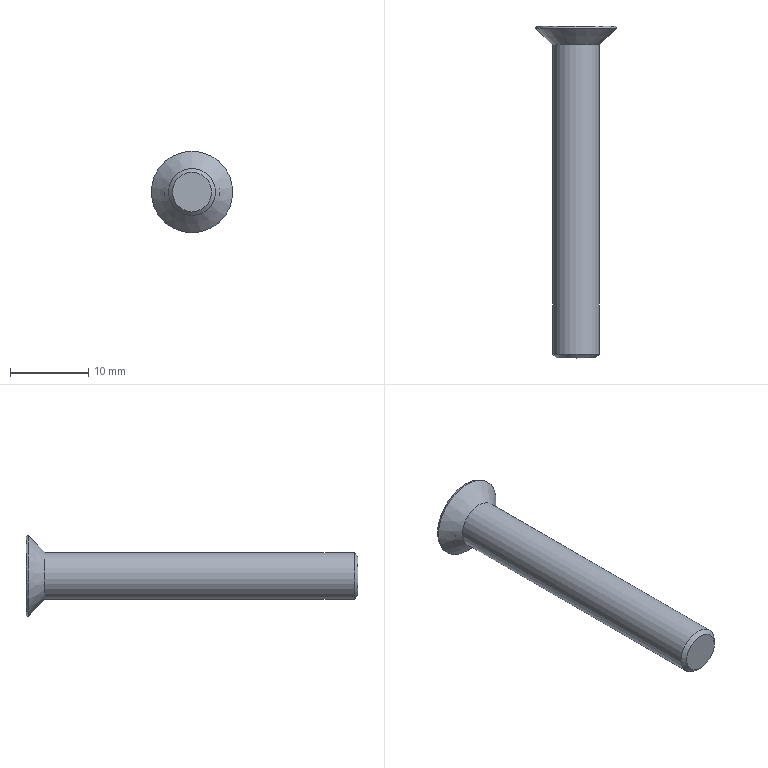Part | STEP file | SD30640 | 1 solid | 23 faces | box 10.421 x 42.38 x 10.421 mm | volume 1245 mm3 | plane 15 | cylinder 5 | cone 3 | commonest cylinder face diameters 0.4 x4 6 x1
STEP:
#1=CARTESIAN_POINT('',(0.,1.224,5.21));
#2=VERTEX_POINT('',#1);
#3=CARTESIAN_POINT('',(0.,1.224,0.));
#4=DIRECTION('',(0.,1.,0.));
#5=DIRECTION('',(0.,0.,1.));
#6=AXIS2_PLACEMENT_3D('',#3,#4,#5);
#7=CIRCLE('',#6,5.21);
#8=EDGE_CURVE('',#2,#2,#7,.T.);
#9=ORIENTED_EDGE('',*,*,#8,.F.);
#10=EDGE_LOOP('',(#9));
#11=FACE_OUTER_BOUND('',#10,.T.);
#12=CARTESIAN_POINT('',(0.,-0.88,-3.));
#13=VERTEX_POINT('',#12);
#14=CARTESIAN_POINT('',(0.,-0.88,0.));
#15=DIRECTION('',(0.,-1.,0.));
#16=DIRECTION('',(0.,0.,-1.));
#17=AXIS2_PLACEMENT_3D('',#14,#15,#16);
#18=CIRCLE('',#17,3.);
#19=EDGE_CURVE('',#13,#13,#18,.T.);
#20=ORIENTED_EDGE('',*,*,#19,.F.);
#21=EDGE_LOOP('',(#20));
#22=FACE_BOUND('',#21,.T.);
#23=CARTESIAN_POINT('',(0.,-0.88,0.));
#24=DIRECTION('',(0.,1.,0.));
#25=DIRECTION('',(0.,0.,1.));
#26=AXIS2_PLACEMENT_3D('',#23,#24,#25);
#27=CONICAL_SURFACE('',#26,3.,0.81);
#28=ADVANCED_FACE('',(#11,#22),#27,.T.);
#29=CARTESIAN_POINT('',(0.,1.5,5.1));
#30=VERTEX_POINT('',#29);
#31=CARTESIAN_POINT('',(0.,1.5,0.));
#32=DIRECTION('',(0.,1.,0.));
#33=DIRECTION('',(0.,0.,1.));
#34=AXIS2_PLACEMENT_3D('',#31,#32,#33);
#35=CIRCLE('',#34,5.1);
#36=EDGE_CURVE('',#30,#30,#35,.T.);
#37=ORIENTED_EDGE('',*,*,#36,.F.);
#38=EDGE_LOOP('',(#37));
#39=FACE_BOUND('',#38,.T.);
#40=ORIENTED_EDGE('',*,*,#8,.T.);
#41=EDGE_LOOP('',(#40));
#42=FACE_OUTER_BOUND('',#41,.T.);
#43=CARTESIAN_POINT('',(0.,1.224,0.));
#44=DIRECTION('',(0.,-1.,0.));
#45=DIRECTION('',(0.,0.,-1.));
#46=AXIS2_PLACEMENT_3D('',#43,#44,#45);
#47=CONICAL_SURFACE('',#46,5.21,0.3804);
#48=ADVANCED_FACE('',(#39,#42),#47,.T.);
#49=CARTESIAN_POINT('',(0.5,1.5,-3.));
#50=VERTEX_POINT('',#49);
#51=CARTESIAN_POINT('',(0.5,1.5,-0.7));
#52=VERTEX_POINT('',#51);
#53=CARTESIAN_POINT('',(0.5,1.5,0.));
#54=DIRECTION('',(0.,0.,1.));
#55=VECTOR('',#54,1000.);
#56=LINE('',#53,#55);
#57=EDGE_CURVE('',#50,#52,#56,.T.);
#58=ORIENTED_EDGE('',*,*,#57,.T.);
#59=CARTESIAN_POINT('',(0.7,1.5,-0.5));
#60=VERTEX_POINT('',#59);
#61=CARTESIAN_POINT('',(0.7,1.5,-0.7));
#62=DIRECTION('',(0.,1.,0.));
#63=DIRECTION('',(0.,0.,-1.));
#64=AXIS2_PLACEMENT_3D('',#61,#62,#63);
#65=CIRCLE('',#64,0.2);
#66=EDGE_CURVE('',#52,#60,#65,.T.);
#67=ORIENTED_EDGE('',*,*,#66,.T.);
#68=CARTESIAN_POINT('',(3.5,1.5,-0.5));
#69=VERTEX_POINT('',#68);
#70=CARTESIAN_POINT('',(5.1,1.5,-0.5));
#71=DIRECTION('',(1.,0.,0.));
#72=VECTOR('',#71,1000.);
#73=LINE('',#70,#72);
#74=EDGE_CURVE('',#60,#69,#73,.T.);
#75=ORIENTED_EDGE('',*,*,#74,.T.);
#76=CARTESIAN_POINT('',(3.5,1.5,0.5));
#77=VERTEX_POINT('',#76);
#78=CARTESIAN_POINT('',(3.5,1.5,0.));
#79=DIRECTION('',(0.,0.,1.));
#80=VECTOR('',#79,1000.);
#81=LINE('',#78,#80);
#82=EDGE_CURVE('',#69,#77,#81,.T.);
#83=ORIENTED_EDGE('',*,*,#82,.T.);
#84=CARTESIAN_POINT('',(0.7,1.5,0.5));
#85=VERTEX_POINT('',#84);
#86=CARTESIAN_POINT('',(5.1,1.5,0.5));
#87=DIRECTION('',(-1.,0.,0.));
#88=VECTOR('',#87,1000.);
#89=LINE('',#86,#88);
#90=EDGE_CURVE('',#77,#85,#89,.T.);
#91=ORIENTED_EDGE('',*,*,#90,.T.);
#92=CARTESIAN_POINT('',(0.5,1.5,0.7));
#93=VERTEX_POINT('',#92);
#94=CARTESIAN_POINT('',(0.7,1.5,0.7));
#95=DIRECTION('',(0.,1.,0.));
#96=DIRECTION('',(0.,0.,-1.));
#97=AXIS2_PLACEMENT_3D('',#94,#95,#96);
#98=CIRCLE('',#97,0.2);
#99=EDGE_CURVE('',#85,#93,#98,.T.);
#100=ORIENTED_EDGE('',*,*,#99,.T.);
#101=CARTESIAN_POINT('',(0.5,1.5,3.));
#102=VERTEX_POINT('',#101);
#103=CARTESIAN_POINT('',(0.5,1.5,0.));
#104=DIRECTION('',(0.,0.,1.));
#105=VECTOR('',#104,1000.);
#106=LINE('',#103,#105);
#107=EDGE_CURVE('',#93,#102,#106,.T.);
#108=ORIENTED_EDGE('',*,*,#107,.T.);
#109=CARTESIAN_POINT('',(-0.5,1.5,3.));
#110=VERTEX_POINT('',#109);
#111=CARTESIAN_POINT('',(5.1,1.5,3.));
#112=DIRECTION('',(-1.,0.,0.));
#113=VECTOR('',#112,1000.);
#114=LINE('',#111,#113);
#115=EDGE_CURVE('',#102,#110,#114,.T.);
#116=ORIENTED_EDGE('',*,*,#115,.T.);
#117=CARTESIAN_POINT('',(-0.5,1.5,0.7));
#118=VERTEX_POINT('',#117);
#119=CARTESIAN_POINT('',(-0.5,1.5,0.));
#120=DIRECTION('',(0.,0.,-1.));
#121=VECTOR('',#120,1000.);
#122=LINE('',#119,#121);
#123=EDGE_CURVE('',#110,#118,#122,.T.);
#124=ORIENTED_EDGE('',*,*,#123,.T.);
#125=CARTESIAN_POINT('',(-0.7,1.5,0.5));
#126=VERTEX_POINT('',#125);
#127=CARTESIAN_POINT('',(-0.7,1.5,0.7));
#128=DIRECTION('',(0.,1.,0.));
#129=DIRECTION('',(0.,0.,-1.));
#130=AXIS2_PLACEMENT_3D('',#127,#128,#129);
#131=CIRCLE('',#130,0.2);
#132=EDGE_CURVE('',#118,#126,#131,.T.);
#133=ORIENTED_EDGE('',*,*,#132,.T.);
#134=CARTESIAN_POINT('',(-3.5,1.5,0.5));
#135=VERTEX_POINT('',#134);
#136=CARTESIAN_POINT('',(5.1,1.5,0.5));
#137=DIRECTION('',(-1.,0.,0.));
#138=VECTOR('',#137,1000.);
#139=LINE('',#136,#138);
#140=EDGE_CURVE('',#126,#135,#139,.T.);
#141=ORIENTED_EDGE('',*,*,#140,.T.);
#142=CARTESIAN_POINT('',(-3.5,1.5,-0.5));
#143=VERTEX_POINT('',#142);
#144=CARTESIAN_POINT('',(-3.5,1.5,0.));
#145=DIRECTION('',(0.,0.,-1.));
#146=VECTOR('',#145,1000.);
#147=LINE('',#144,#146);
#148=EDGE_CURVE('',#135,#143,#147,.T.);
#149=ORIENTED_EDGE('',*,*,#148,.T.);
#150=CARTESIAN_POINT('',(-0.7,1.5,-0.5));
#151=VERTEX_POINT('',#150);
#152=CARTESIAN_POINT('',(5.1,1.5,-0.5));
#153=DIRECTION('',(1.,0.,0.));
#154=VECTOR('',#153,1000.);
#155=LINE('',#152,#154);
#156=EDGE_CURVE('',#143,#151,#155,.T.);
#157=ORIENTED_EDGE('',*,*,#156,.T.);
#158=CARTESIAN_POINT('',(-0.5,1.5,-0.7));
#159=VERTEX_POINT('',#158);
#160=CARTESIAN_POINT('',(-0.7,1.5,-0.7));
#161=DIRECTION('',(0.,1.,0.));
#162=DIRECTION('',(0.,0.,-1.));
#163=AXIS2_PLACEMENT_3D('',#160,#161,#162);
#164=CIRCLE('',#163,0.2);
#165=EDGE_CURVE('',#151,#159,#164,.T.);
#166=ORIENTED_EDGE('',*,*,#165,.T.);
#167=CARTESIAN_POINT('',(-0.5,1.5,-3.));
#168=VERTEX_POINT('',#167);
#169=CARTESIAN_POINT('',(-0.5,1.5,0.));
#170=DIRECTION('',(0.,0.,-1.));
#171=VECTOR('',#170,1000.);
#172=LINE('',#169,#171);
#173=EDGE_CURVE('',#159,#168,#172,.T.);
#174=ORIENTED_EDGE('',*,*,#173,.T.);
#175=CARTESIAN_POINT('',(5.1,1.5,-3.));
#176=DIRECTION('',(1.,0.,0.));
#177=VECTOR('',#176,1000.);
#178=LINE('',#175,#177);
#179=EDGE_CURVE('',#168,#50,#178,.T.);
#180=ORIENTED_EDGE('',*,*,#179,.T.);
#181=EDGE_LOOP('',(#58,#67,#75,#83,#91,#100,#108,#116,#124,#133,#141,#149,#157,#166,#174,#180));
#182=FACE_BOUND('',#181,.T.);
#183=ORIENTED_EDGE('',*,*,#36,.T.);
#184=EDGE_LOOP('',(#183));
#185=FACE_OUTER_BOUND('',#184,.T.);
#186=CARTESIAN_POINT('',(5.1,1.5,0.));
#187=DIRECTION('',(0.,-1.,0.));
#188=DIRECTION('',(0.,0.,-1.));
#189=AXIS2_PLACEMENT_3D('',#186,#187,#188);
#190=PLANE('',#189);
#191=ADVANCED_FACE('',(#182,#185),#190,.F.);
#192=CARTESIAN_POINT('',(0.5,-0.2,-0.7));
#193=VERTEX_POINT('',#192);
#194=CARTESIAN_POINT('',(0.5,-0.2,-0.7));
#195=DIRECTION('',(0.,1.,0.));
#196=VECTOR('',#195,1000.);
#197=LINE('',#194,#196);
#198=EDGE_CURVE('',#193,#52,#197,.T.);
#199=ORIENTED_EDGE('',*,*,#198,.F.);
#200=CARTESIAN_POINT('',(0.7,-0.2,-0.5));
#201=VERTEX_POINT('',#200);
#202=CARTESIAN_POINT('',(0.7,-0.2,-0.7));
#203=DIRECTION('',(0.,-1.,0.));
#204=DIRECTION('',(0.,0.,-1.));
#205=AXIS2_PLACEMENT_3D('',#202,#203,#204);
#206=CIRCLE('',#205,0.2);
#207=EDGE_CURVE('',#201,#193,#206,.T.);
#208=ORIENTED_EDGE('',*,*,#207,.F.);
#209=CARTESIAN_POINT('',(0.7,-0.2,-0.5));
#210=DIRECTION('',(0.,1.,0.));
#211=VECTOR('',#210,1000.);
#212=LINE('',#209,#211);
#213=EDGE_CURVE('',#201,#60,#212,.T.);
#214=ORIENTED_EDGE('',*,*,#213,.T.);
#215=ORIENTED_EDGE('',*,*,#66,.F.);
#216=EDGE_LOOP('',(#199,#208,#214,#215));
#217=FACE_OUTER_BOUND('',#216,.T.);
#218=CARTESIAN_POINT('',(0.7,-0.2,-0.7));
#219=DIRECTION('',(0.,1.,0.));
#220=DIRECTION('',(0.,0.,1.));
#221=AXIS2_PLACEMENT_3D('',#218,#219,#220);
#222=CYLINDRICAL_SURFACE('',#221,0.2);
#223=ADVANCED_FACE('',(#217),#222,.T.);
#224=ORIENTED_EDGE('',*,*,#213,.F.);
#225=CARTESIAN_POINT('',(3.5,-0.2,-0.5));
#226=VERTEX_POINT('',#225);
#227=CARTESIAN_POINT('',(0.8,-0.2,-0.5));
#228=DIRECTION('',(-1.,0.,0.));
#229=VECTOR('',#228,1000.);
#230=LINE('',#227,#229);
#231=EDGE_CURVE('',#226,#201,#230,.T.);
#232=ORIENTED_EDGE('',*,*,#231,.F.);
#233=CARTESIAN_POINT('',(3.5,-0.2,-0.5));
#234=DIRECTION('',(0.,1.,0.));
#235=VECTOR('',#234,1000.);
#236=LINE('',#233,#235);
#237=EDGE_CURVE('',#226,#69,#236,.T.);
#238=ORIENTED_EDGE('',*,*,#237,.T.);
#239=ORIENTED_EDGE('',*,*,#74,.F.);
#240=EDGE_LOOP('',(#224,#232,#238,#239));
#241=FACE_OUTER_BOUND('',#240,.T.);
#242=CARTESIAN_POINT('',(0.8,-0.2,-0.5));
#243=DIRECTION('',(0.,0.,-1.));
#244=DIRECTION('',(-1.,0.,0.));
#245=AXIS2_PLACEMENT_3D('',#242,#243,#244);
#246=PLANE('',#245);
#247=ADVANCED_FACE('',(#241),#246,.F.);
#248=ORIENTED_EDGE('',*,*,#237,.F.);
#249=CARTESIAN_POINT('',(3.5,-0.2,0.5));
#250=VERTEX_POINT('',#249);
#251=CARTESIAN_POINT('',(3.5,-0.2,0.5));
#252=DIRECTION('',(0.,0.,-1.));
#253=VECTOR('',#252,1000.);
#254=LINE('',#251,#253);
#255=EDGE_CURVE('',#250,#226,#254,.T.);
#256=ORIENTED_EDGE('',*,*,#255,.F.);
#257=CARTESIAN_POINT('',(3.5,-0.2,0.5));
#258=DIRECTION('',(0.,1.,0.));
#259=VECTOR('',#258,1000.);
#260=LINE('',#257,#259);
#261=EDGE_CURVE('',#250,#77,#260,.T.);
#262=ORIENTED_EDGE('',*,*,#261,.T.);
#263=ORIENTED_EDGE('',*,*,#82,.F.);
#264=EDGE_LOOP('',(#248,#256,#262,#263));
#265=FACE_OUTER_BOUND('',#264,.T.);
#266=CARTESIAN_POINT('',(3.5,-0.2,0.5));
#267=DIRECTION('',(1.,0.,0.));
#268=DIRECTION('',(0.,0.,-1.));
#269=AXIS2_PLACEMENT_3D('',#266,#267,#268);
#270=PLANE('',#269);
#271=ADVANCED_FACE('',(#265),#270,.F.);
#272=ORIENTED_EDGE('',*,*,#261,.F.);
#273=CARTESIAN_POINT('',(0.7,-0.2,0.5));
#274=VERTEX_POINT('',#273);
#275=CARTESIAN_POINT('',(0.7,-0.2,0.5));
#276=DIRECTION('',(1.,0.,0.));
#277=VECTOR('',#276,1000.);
#278=LINE('',#275,#277);
#279=EDGE_CURVE('',#274,#250,#278,.T.);
#280=ORIENTED_EDGE('',*,*,#279,.F.);
#281=CARTESIAN_POINT('',(0.7,-0.2,0.5));
#282=DIRECTION('',(0.,1.,0.));
#283=VECTOR('',#282,1000.);
#284=LINE('',#281,#283);
#285=EDGE_CURVE('',#274,#85,#284,.T.);
#286=ORIENTED_EDGE('',*,*,#285,.T.);
#287=ORIENTED_EDGE('',*,*,#90,.F.);
#288=EDGE_LOOP('',(#272,#280,#286,#287));
#289=FACE_OUTER_BOUND('',#288,.T.);
#290=CARTESIAN_POINT('',(0.7,-0.2,0.5));
#291=DIRECTION('',(0.,0.,1.));
#292=DIRECTION('',(1.,0.,0.));
#293=AXIS2_PLACEMENT_3D('',#290,#291,#292);
#294=PLANE('',#293);
#295=ADVANCED_FACE('',(#289),#294,.F.);
#296=ORIENTED_EDGE('',*,*,#285,.F.);
#297=CARTESIAN_POINT('',(0.5,-0.2,0.7));
#298=VERTEX_POINT('',#297);
#299=CARTESIAN_POINT('',(0.7,-0.2,0.7));
#300=DIRECTION('',(0.,-1.,0.));
#301=DIRECTION('',(0.,0.,1.));
#302=AXIS2_PLACEMENT_3D('',#299,#300,#301);
#303=CIRCLE('',#302,0.2);
#304=EDGE_CURVE('',#298,#274,#303,.T.);
#305=ORIENTED_EDGE('',*,*,#304,.F.);
#306=CARTESIAN_POINT('',(0.5,-0.2,0.7));
#307=DIRECTION('',(0.,1.,0.));
#308=VECTOR('',#307,1000.);
#309=LINE('',#306,#308);
#310=EDGE_CURVE('',#298,#93,#309,.T.);
#311=ORIENTED_EDGE('',*,*,#310,.T.);
#312=ORIENTED_EDGE('',*,*,#99,.F.);
#313=EDGE_LOOP('',(#296,#305,#311,#312));
#314=FACE_OUTER_BOUND('',#313,.T.);
#315=CARTESIAN_POINT('',(0.7,-0.2,0.7));
#316=DIRECTION('',(0.,1.,0.));
#317=DIRECTION('',(0.,0.,1.));
#318=AXIS2_PLACEMENT_3D('',#315,#316,#317);
#319=CYLINDRICAL_SURFACE('',#318,0.2);
#320=ADVANCED_FACE('',(#314),#319,.T.);
#321=ORIENTED_EDGE('',*,*,#310,.F.);
#322=CARTESIAN_POINT('',(0.5,-0.2,3.));
#323=VERTEX_POINT('',#322);
#324=CARTESIAN_POINT('',(0.5,-0.2,3.));
#325=DIRECTION('',(0.,0.,-1.));
#326=VECTOR('',#325,1000.);
#327=LINE('',#324,#326);
#328=EDGE_CURVE('',#323,#298,#327,.T.);
#329=ORIENTED_EDGE('',*,*,#328,.F.);
#330=CARTESIAN_POINT('',(0.5,-0.2,3.));
#331=DIRECTION('',(0.,1.,0.));
#332=VECTOR('',#331,1000.);
#333=LINE('',#330,#332);
#334=EDGE_CURVE('',#323,#102,#333,.T.);
#335=ORIENTED_EDGE('',*,*,#334,.T.);
#336=ORIENTED_EDGE('',*,*,#107,.F.);
#337=EDGE_LOOP('',(#321,#329,#335,#336));
#338=FACE_OUTER_BOUND('',#337,.T.);
#339=CARTESIAN_POINT('',(0.5,-0.2,3.));
#340=DIRECTION('',(1.,0.,0.));
#341=DIRECTION('',(0.,0.,-1.));
#342=AXIS2_PLACEMENT_3D('',#339,#340,#341);
#343=PLANE('',#342);
#344=ADVANCED_FACE('',(#338),#343,.F.);
#345=ORIENTED_EDGE('',*,*,#334,.F.);
#346=CARTESIAN_POINT('',(-0.5,-0.2,3.));
#347=VERTEX_POINT('',#346);
#348=CARTESIAN_POINT('',(-0.5,-0.2,3.));
#349=DIRECTION('',(1.,0.,0.));
#350=VECTOR('',#349,1000.);
#351=LINE('',#348,#350);
#352=EDGE_CURVE('',#347,#323,#351,.T.);
#353=ORIENTED_EDGE('',*,*,#352,.F.);
#354=CARTESIAN_POINT('',(-0.5,-0.2,3.));
#355=DIRECTION('',(0.,1.,0.));
#356=VECTOR('',#355,1000.);
#357=LINE('',#354,#356);
#358=EDGE_CURVE('',#347,#110,#357,.T.);
#359=ORIENTED_EDGE('',*,*,#358,.T.);
#360=ORIENTED_EDGE('',*,*,#115,.F.);
#361=EDGE_LOOP('',(#345,#353,#359,#360));
#362=FACE_OUTER_BOUND('',#361,.T.);
#363=CARTESIAN_POINT('',(-0.5,-0.2,3.));
#364=DIRECTION('',(0.,0.,1.));
#365=DIRECTION('',(1.,0.,0.));
#366=AXIS2_PLACEMENT_3D('',#363,#364,#365);
#367=PLANE('',#366);
#368=ADVANCED_FACE('',(#362),#367,.F.);
#369=ORIENTED_EDGE('',*,*,#358,.F.);
#370=CARTESIAN_POINT('',(-0.5,-0.2,0.7));
#371=VERTEX_POINT('',#370);
#372=CARTESIAN_POINT('',(-0.5,-0.2,3.));
#373=DIRECTION('',(0.,0.,1.));
#374=VECTOR('',#373,1000.);
#375=LINE('',#372,#374);
#376=EDGE_CURVE('',#371,#347,#375,.T.);
#377=ORIENTED_EDGE('',*,*,#376,.F.);
#378=CARTESIAN_POINT('',(-0.5,-0.2,0.7));
#379=DIRECTION('',(0.,1.,0.));
#380=VECTOR('',#379,1000.);
#381=LINE('',#378,#380);
#382=EDGE_CURVE('',#371,#118,#381,.T.);
#383=ORIENTED_EDGE('',*,*,#382,.T.);
#384=ORIENTED_EDGE('',*,*,#123,.F.);
#385=EDGE_LOOP('',(#369,#377,#383,#384));
#386=FACE_OUTER_BOUND('',#385,.T.);
#387=CARTESIAN_POINT('',(-0.5,-0.2,3.));
#388=DIRECTION('',(-1.,0.,0.));
#389=DIRECTION('',(0.,0.,1.));
#390=AXIS2_PLACEMENT_3D('',#387,#388,#389);
#391=PLANE('',#390);
#392=ADVANCED_FACE('',(#386),#391,.F.);
#393=ORIENTED_EDGE('',*,*,#382,.F.);
#394=CARTESIAN_POINT('',(-0.7,-0.2,0.5));
#395=VERTEX_POINT('',#394);
#396=CARTESIAN_POINT('',(-0.7,-0.2,0.7));
#397=DIRECTION('',(0.,-1.,0.));
#398=DIRECTION('',(0.,0.,1.));
#399=AXIS2_PLACEMENT_3D('',#396,#397,#398);
#400=CIRCLE('',#399,0.2);
#401=EDGE_CURVE('',#395,#371,#400,.T.);
#402=ORIENTED_EDGE('',*,*,#401,.F.);
#403=CARTESIAN_POINT('',(-0.7,-0.2,0.5));
#404=DIRECTION('',(0.,1.,0.));
#405=VECTOR('',#404,1000.);
#406=LINE('',#403,#405);
#407=EDGE_CURVE('',#395,#126,#406,.T.);
#408=ORIENTED_EDGE('',*,*,#407,.T.);
#409=ORIENTED_EDGE('',*,*,#132,.F.);
#410=EDGE_LOOP('',(#393,#402,#408,#409));
#411=FACE_OUTER_BOUND('',#410,.T.);
#412=CARTESIAN_POINT('',(-0.7,-0.2,0.7));
#413=DIRECTION('',(0.,1.,0.));
#414=DIRECTION('',(0.,0.,1.));
#415=AXIS2_PLACEMENT_3D('',#412,#413,#414);
#416=CYLINDRICAL_SURFACE('',#415,0.2);
#417=ADVANCED_FACE('',(#411),#416,.T.);
#418=ORIENTED_EDGE('',*,*,#407,.F.);
#419=CARTESIAN_POINT('',(-3.5,-0.2,0.5));
#420=VERTEX_POINT('',#419);
#421=CARTESIAN_POINT('',(-0.7,-0.2,0.5));
#422=DIRECTION('',(1.,0.,0.));
#423=VECTOR('',#422,1000.);
#424=LINE('',#421,#423);
#425=EDGE_CURVE('',#420,#395,#424,.T.);
#426=ORIENTED_EDGE('',*,*,#425,.F.);
#427=CARTESIAN_POINT('',(-3.5,-0.2,0.5));
#428=DIRECTION('',(0.,1.,0.));
#429=VECTOR('',#428,1000.);
#430=LINE('',#427,#429);
#431=EDGE_CURVE('',#420,#135,#430,.T.);
#432=ORIENTED_EDGE('',*,*,#431,.T.);
#433=ORIENTED_EDGE('',*,*,#140,.F.);
#434=EDGE_LOOP('',(#418,#426,#432,#433));
#435=FACE_OUTER_BOUND('',#434,.T.);
#436=CARTESIAN_POINT('',(-0.7,-0.2,0.5));
#437=DIRECTION('',(0.,0.,1.));
#438=DIRECTION('',(1.,0.,0.));
#439=AXIS2_PLACEMENT_3D('',#436,#437,#438);
#440=PLANE('',#439);
#441=ADVANCED_FACE('',(#435),#440,.F.);
#442=ORIENTED_EDGE('',*,*,#431,.F.);
#443=CARTESIAN_POINT('',(-3.5,-0.2,-0.5));
#444=VERTEX_POINT('',#443);
#445=CARTESIAN_POINT('',(-3.5,-0.2,0.5));
#446=DIRECTION('',(0.,0.,1.));
#447=VECTOR('',#446,1000.);
#448=LINE('',#445,#447);
#449=EDGE_CURVE('',#444,#420,#448,.T.);
#450=ORIENTED_EDGE('',*,*,#449,.F.);
#451=CARTESIAN_POINT('',(-3.5,-0.2,-0.5));
#452=DIRECTION('',(0.,1.,0.));
#453=VECTOR('',#452,1000.);
#454=LINE('',#451,#453);
#455=EDGE_CURVE('',#444,#143,#454,.T.);
#456=ORIENTED_EDGE('',*,*,#455,.T.);
#457=ORIENTED_EDGE('',*,*,#148,.F.);
#458=EDGE_LOOP('',(#442,#450,#456,#457));
#459=FACE_OUTER_BOUND('',#458,.T.);
#460=CARTESIAN_POINT('',(-3.5,-0.2,0.5));
#461=DIRECTION('',(-1.,0.,0.));
#462=DIRECTION('',(0.,0.,1.));
#463=AXIS2_PLACEMENT_3D('',#460,#461,#462);
#464=PLANE('',#463);
#465=ADVANCED_FACE('',(#459),#464,.F.);
#466=ORIENTED_EDGE('',*,*,#455,.F.);
#467=CARTESIAN_POINT('',(-0.7,-0.2,-0.5));
#468=VERTEX_POINT('',#467);
#469=CARTESIAN_POINT('',(-0.7,-0.2,-0.5));
#470=DIRECTION('',(-1.,0.,0.));
#471=VECTOR('',#470,1000.);
#472=LINE('',#469,#471);
#473=EDGE_CURVE('',#468,#444,#472,.T.);
#474=ORIENTED_EDGE('',*,*,#473,.F.);
#475=CARTESIAN_POINT('',(-0.7,-0.2,-0.5));
#476=DIRECTION('',(0.,1.,0.));
#477=VECTOR('',#476,1000.);
#478=LINE('',#475,#477);
#479=EDGE_CURVE('',#468,#151,#478,.T.);
#480=ORIENTED_EDGE('',*,*,#479,.T.);
#481=ORIENTED_EDGE('',*,*,#156,.F.);
#482=EDGE_LOOP('',(#466,#474,#480,#481));
#483=FACE_OUTER_BOUND('',#482,.T.);
#484=CARTESIAN_POINT('',(-0.7,-0.2,-0.5));
#485=DIRECTION('',(0.,0.,-1.));
#486=DIRECTION('',(-1.,0.,0.));
#487=AXIS2_PLACEMENT_3D('',#484,#485,#486);
#488=PLANE('',#487);
#489=ADVANCED_FACE('',(#483),#488,.F.);
#490=ORIENTED_EDGE('',*,*,#479,.F.);
#491=CARTESIAN_POINT('',(-0.5,-0.2,-0.7));
#492=VERTEX_POINT('',#491);
#493=CARTESIAN_POINT('',(-0.7,-0.2,-0.7));
#494=DIRECTION('',(0.,-1.,0.));
#495=DIRECTION('',(0.,0.,-1.));
#496=AXIS2_PLACEMENT_3D('',#493,#494,#495);
#497=CIRCLE('',#496,0.2);
#498=EDGE_CURVE('',#492,#468,#497,.T.);
#499=ORIENTED_EDGE('',*,*,#498,.F.);
#500=CARTESIAN_POINT('',(-0.5,-0.2,-0.7));
#501=DIRECTION('',(0.,1.,0.));
#502=VECTOR('',#501,1000.);
#503=LINE('',#500,#502);
#504=EDGE_CURVE('',#492,#159,#503,.T.);
#505=ORIENTED_EDGE('',*,*,#504,.T.);
#506=ORIENTED_EDGE('',*,*,#165,.F.);
#507=EDGE_LOOP('',(#490,#499,#505,#506));
#508=FACE_OUTER_BOUND('',#507,.T.);
#509=CARTESIAN_POINT('',(-0.7,-0.2,-0.7));
#510=DIRECTION('',(0.,1.,0.));
#511=DIRECTION('',(0.,0.,1.));
#512=AXIS2_PLACEMENT_3D('',#509,#510,#511);
#513=CYLINDRICAL_SURFACE('',#512,0.2);
#514=ADVANCED_FACE('',(#508),#513,.T.);
#515=ORIENTED_EDGE('',*,*,#504,.F.);
#516=CARTESIAN_POINT('',(-0.5,-0.2,-3.));
#517=VERTEX_POINT('',#516);
#518=CARTESIAN_POINT('',(-0.5,-0.2,-3.));
#519=DIRECTION('',(0.,0.,1.));
#520=VECTOR('',#519,1000.);
#521=LINE('',#518,#520);
#522=EDGE_CURVE('',#517,#492,#521,.T.);
#523=ORIENTED_EDGE('',*,*,#522,.F.);
#524=CARTESIAN_POINT('',(-0.5,-0.2,-3.));
#525=DIRECTION('',(0.,1.,0.));
#526=VECTOR('',#525,1000.);
#527=LINE('',#524,#526);
#528=EDGE_CURVE('',#517,#168,#527,.T.);
#529=ORIENTED_EDGE('',*,*,#528,.T.);
#530=ORIENTED_EDGE('',*,*,#173,.F.);
#531=EDGE_LOOP('',(#515,#523,#529,#530));
#532=FACE_OUTER_BOUND('',#531,.T.);
#533=CARTESIAN_POINT('',(-0.5,-0.2,-3.));
#534=DIRECTION('',(-1.,0.,0.));
#535=DIRECTION('',(0.,0.,1.));
#536=AXIS2_PLACEMENT_3D('',#533,#534,#535);
#537=PLANE('',#536);
#538=ADVANCED_FACE('',(#532),#537,.F.);
#539=ORIENTED_EDGE('',*,*,#528,.F.);
#540=CARTESIAN_POINT('',(0.5,-0.2,-3.));
#541=VERTEX_POINT('',#540);
#542=CARTESIAN_POINT('',(-0.5,-0.2,-3.));
#543=DIRECTION('',(-1.,0.,0.));
#544=VECTOR('',#543,1000.);
#545=LINE('',#542,#544);
#546=EDGE_CURVE('',#541,#517,#545,.T.);
#547=ORIENTED_EDGE('',*,*,#546,.F.);
#548=CARTESIAN_POINT('',(0.5,-0.2,-3.));
#549=DIRECTION('',(0.,1.,0.));
#550=VECTOR('',#549,1000.);
#551=LINE('',#548,#550);
#552=EDGE_CURVE('',#541,#50,#551,.T.);
#553=ORIENTED_EDGE('',*,*,#552,.T.);
#554=ORIENTED_EDGE('',*,*,#179,.F.);
#555=EDGE_LOOP('',(#539,#547,#553,#554));
#556=FACE_OUTER_BOUND('',#555,.T.);
#557=CARTESIAN_POINT('',(-0.5,-0.2,-3.));
#558=DIRECTION('',(0.,0.,-1.));
#559=DIRECTION('',(-1.,0.,0.));
#560=AXIS2_PLACEMENT_3D('',#557,#558,#559);
#561=PLANE('',#560);
#562=ADVANCED_FACE('',(#556),#561,.F.);
#563=ORIENTED_EDGE('',*,*,#552,.F.);
#564=CARTESIAN_POINT('',(0.5,-0.2,-3.));
#565=DIRECTION('',(0.,0.,-1.));
#566=VECTOR('',#565,1000.);
#567=LINE('',#564,#566);
#568=EDGE_CURVE('',#193,#541,#567,.T.);
#569=ORIENTED_EDGE('',*,*,#568,.F.);
#570=ORIENTED_EDGE('',*,*,#198,.T.);
#571=ORIENTED_EDGE('',*,*,#57,.F.);
#572=EDGE_LOOP('',(#563,#569,#570,#571));
#573=FACE_OUTER_BOUND('',#572,.T.);
#574=CARTESIAN_POINT('',(0.5,-0.2,-3.));
#575=DIRECTION('',(1.,0.,0.));
#576=DIRECTION('',(0.,0.,-1.));
#577=AXIS2_PLACEMENT_3D('',#574,#575,#576);
#578=PLANE('',#577);
#579=ADVANCED_FACE('',(#573),#578,.F.);
#580=ORIENTED_EDGE('',*,*,#207,.T.);
#581=ORIENTED_EDGE('',*,*,#568,.T.);
#582=ORIENTED_EDGE('',*,*,#546,.T.);
#583=ORIENTED_EDGE('',*,*,#522,.T.);
#584=ORIENTED_EDGE('',*,*,#498,.T.);
#585=ORIENTED_EDGE('',*,*,#473,.T.);
#586=ORIENTED_EDGE('',*,*,#449,.T.);
#587=ORIENTED_EDGE('',*,*,#425,.T.);
#588=ORIENTED_EDGE('',*,*,#401,.T.);
#589=ORIENTED_EDGE('',*,*,#376,.T.);
#590=ORIENTED_EDGE('',*,*,#352,.T.);
#591=ORIENTED_EDGE('',*,*,#328,.T.);
#592=ORIENTED_EDGE('',*,*,#304,.T.);
#593=ORIENTED_EDGE('',*,*,#279,.T.);
#594=ORIENTED_EDGE('',*,*,#255,.T.);
#595=ORIENTED_EDGE('',*,*,#231,.T.);
#596=EDGE_LOOP('',(#580,#581,#582,#583,#584,#585,#586,#587,#588,#589,#590,#591,#592,#593,#594,#595));
#597=FACE_OUTER_BOUND('',#596,.T.);
#598=CARTESIAN_POINT('',(0.7,-0.2,-0.7));
#599=DIRECTION('',(0.,-1.,0.));
#600=DIRECTION('',(0.,0.,-1.));
#601=AXIS2_PLACEMENT_3D('',#598,#599,#600);
#602=PLANE('',#601);
#603=ADVANCED_FACE('',(#597),#602,.F.);
#604=CARTESIAN_POINT('',(0.,-40.38,-3.));
#605=VERTEX_POINT('',#604);
#606=CARTESIAN_POINT('',(0.,-40.38,0.));
#607=DIRECTION('',(0.,1.,0.));
#608=DIRECTION('',(0.,0.,-1.));
#609=AXIS2_PLACEMENT_3D('',#606,#607,#608);
#610=CIRCLE('',#609,3.);
#611=EDGE_CURVE('',#605,#605,#610,.T.);
#612=ORIENTED_EDGE('',*,*,#611,.T.);
#613=EDGE_LOOP('',(#612));
#614=FACE_OUTER_BOUND('',#613,.T.);
#615=ORIENTED_EDGE('',*,*,#19,.T.);
#616=EDGE_LOOP('',(#615));
#617=FACE_OUTER_BOUND('',#616,.T.);
#618=CARTESIAN_POINT('',(0.,-40.88,0.));
#619=DIRECTION('',(0.,1.,0.));
#620=DIRECTION('',(0.,0.,1.));
#621=AXIS2_PLACEMENT_3D('',#618,#619,#620);
#622=CYLINDRICAL_SURFACE('',#621,3.);
#623=ADVANCED_FACE('',(#614,#617),#622,.T.);
#624=CARTESIAN_POINT('',(0.,-40.88,-2.5));
#625=VERTEX_POINT('',#624);
#626=CARTESIAN_POINT('',(0.,-40.88,0.));
#627=DIRECTION('',(0.,-1.,0.));
#628=DIRECTION('',(0.,0.,-1.));
#629=AXIS2_PLACEMENT_3D('',#626,#627,#628);
#630=CIRCLE('',#629,2.5);
#631=EDGE_CURVE('',#625,#625,#630,.T.);
#632=ORIENTED_EDGE('',*,*,#631,.T.);
#633=EDGE_LOOP('',(#632));
#634=FACE_OUTER_BOUND('',#633,.T.);
#635=CARTESIAN_POINT('',(0.,-40.88,0.));
#636=DIRECTION('',(0.,-1.,0.));
#637=DIRECTION('',(0.,0.,-1.));
#638=AXIS2_PLACEMENT_3D('',#635,#636,#637);
#639=PLANE('',#638);
#640=ADVANCED_FACE('',(#634),#639,.T.);
#641=ORIENTED_EDGE('',*,*,#611,.F.);
#642=EDGE_LOOP('',(#641));
#643=FACE_OUTER_BOUND('',#642,.T.);
#644=ORIENTED_EDGE('',*,*,#631,.F.);
#645=EDGE_LOOP('',(#644));
#646=FACE_BOUND('',#645,.T.);
#647=CARTESIAN_POINT('',(0.,-40.88,0.));
#648=DIRECTION('',(0.,1.,0.));
#649=DIRECTION('',(0.,0.,1.));
#650=AXIS2_PLACEMENT_3D('',#647,#648,#649);
#651=CONICAL_SURFACE('',#650,2.5,0.7854);
#652=ADVANCED_FACE('',(#643,#646),#651,.T.);
#653=CLOSED_SHELL('',(#28,#48,#191,#223,#247,#271,#295,#320,#344,#368,#392,#417,#441,#465,#489,#514,#538,#562,#579,#603,#623,#640,#652));
#654=MANIFOLD_SOLID_BREP('',#653);
#655=CARTESIAN_POINT('',(0.,0.,0.));
#656=DIRECTION('',(0.,0.,1.));
#657=DIRECTION('',(1.,0.,0.));
#658=AXIS2_PLACEMENT_3D('',#655,#656,#657);
#659=(LENGTH_UNIT()NAMED_UNIT(*)SI_UNIT(.MILLI.,.METRE.));
#660=UNCERTAINTY_MEASURE_WITH_UNIT(LENGTH_MEASURE(0.00001),#659,'','');
#661=(NAMED_UNIT(*)PLANE_ANGLE_UNIT()SI_UNIT($,.RADIAN.));
#662=(NAMED_UNIT(*)SI_UNIT($,.STERADIAN.)SOLID_ANGLE_UNIT());
#663=(GEOMETRIC_REPRESENTATION_CONTEXT(3)GLOBAL_UNCERTAINTY_ASSIGNED_CONTEXT((#660))GLOBAL_UNIT_ASSIGNED_CONTEXT((#659,#661,#662))REPRESENTATION_CONTEXT('',''));
#664=ADVANCED_BREP_SHAPE_REPRESENTATION('',(#654,#658),#663);